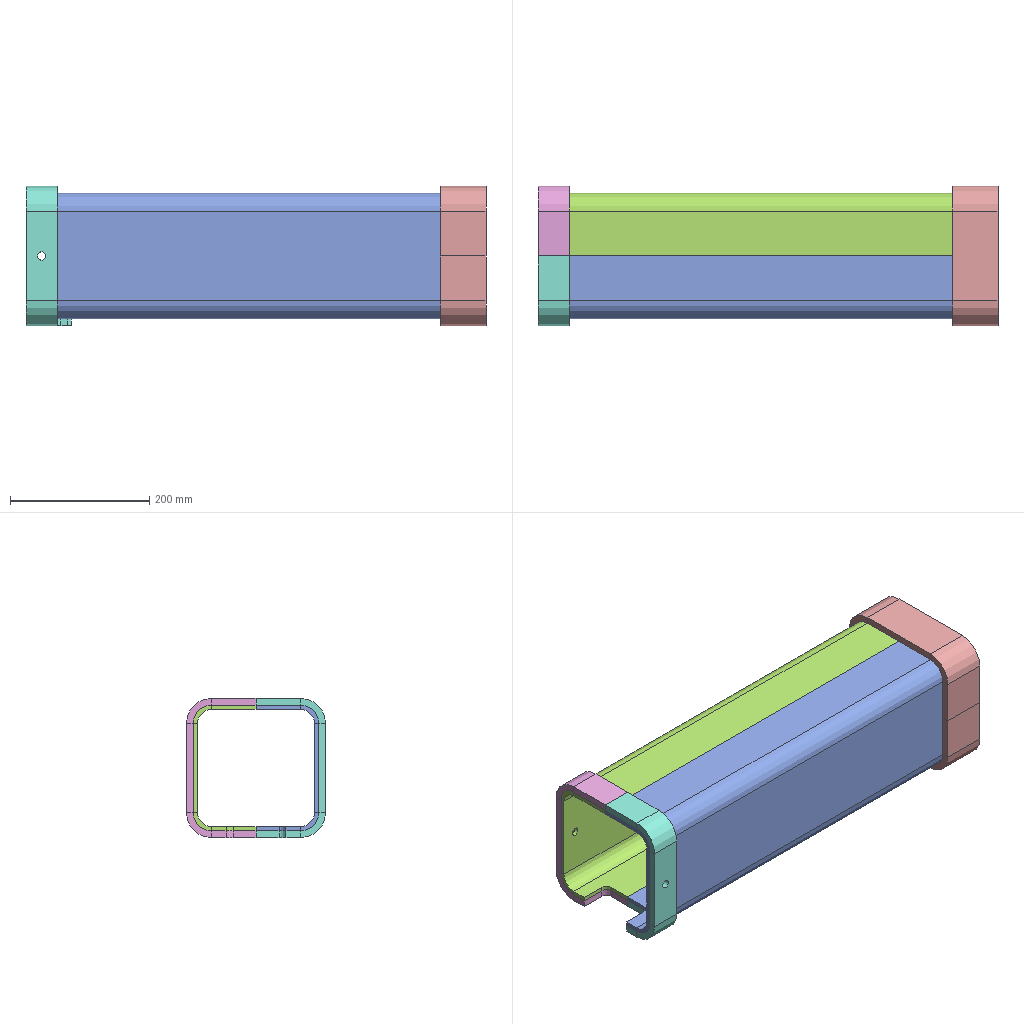Assembly | SolidWorks | 5 different items | 6 placed | box 660 x 200 x 200 mm
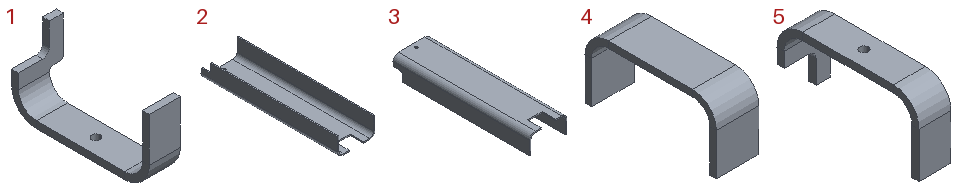Parts list (item | quantity | size | volume | features):
1 | x1 | 65 x 200.003 x 99.994 mm | 150355 mm3 | features Cut 1, FlatPattern 1, SM3dBend 1, SMBaseFlange 1, SheetMetal 1
2 | x1 | 180.012 x 660 x 89.996 mm | 1260450 mm3 | features Cut 1, FlatPattern 1, SM3dBend 1, SMBaseFlange 1, SheetMetal 1
3 | x1 | 180.012 x 660 x 89.996 mm | 1260450 mm3 | features Cut 1, FlatPattern 1, SM3dBend 1, SMBaseFlange 1, SheetMetal 1
4 | x2 | 65 x 200.003 x 99.994 mm | 229697 mm3 | features FlatPattern 1, SM3dBend 1, SMBaseFlange 1, SheetMetal 1
5 | x1 | 65 x 200.003 x 99.994 mm | 150355 mm3 | features Cut 1, FlatPattern 1, SM3dBend 1, SMBaseFlange 1, SheetMetal 1
Mates (type | each side: item.copy, entity, surface, feature):
Coincident | 4.1 face plane Base-Flange1 | 4.2 face plane Base-Flange1 | 2 times
Coincident | 4.1 face plane Sketched Bend1 | 4.2 face plane Sketched Bend1
Coincident | 4.1 face plane Sketched Bend1 | 3.1 face plane Base-Flange1
Coincident | 4.1 face plane Base-Flange1 | 3.1 face plane Sketched Bend1
Coincident | 4.2 face plane Base-Flange1 | 3.1 face plane Base-Flange1
Coincident | 3.1 face plane Sketched Bend1 | 2.1 face plane Sketched Bend1
Coincident | 3.1 face plane Base-Flange1 | 2.1 face plane Base-Flange1 | 2 times
Coincident | 2.1 face plane Base-Flange1 | 5.1 face plane Base-Flange1
Coincident | 2.1 face plane Sketched Bend1 | 5.1 face plane Sketched Bend1
Coincident | 2.1 face plane Base-Flange1 | 5.1 face plane Sketch Bend2
Coincident | 5.1 face plane Base-Flange1 | 1.1 face plane Base-Flange1 | 2 times
Coincident | 5.1 face plane Sketched Bend1 | 1.1 face plane Sketched Bend2